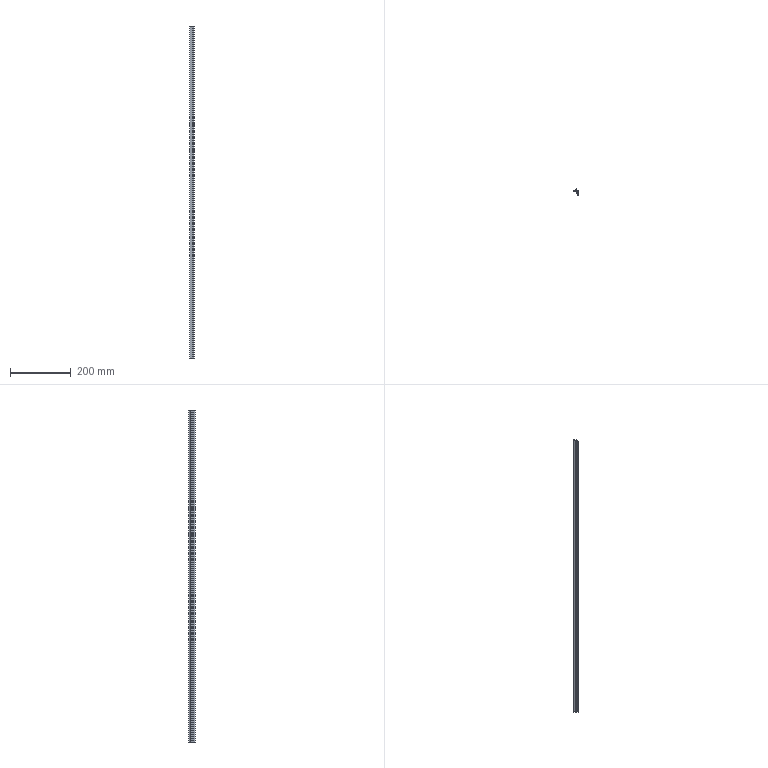Part | SolidWorks | features BaseBody 1, ICE 1, MoveFace 1 | 1 solid | 27 faces | box 14 x 20.3 x 1090 mm | volume 55498 mm3 | plane 20 | cylinder 7 | commonest cylinder face diameters 0.387 x2 0.8 x2 0.4 x1 20 x1 22 x1
STEP:
#1=CARTESIAN_POINT('',(-5.304,-0.625,200.));
#2=VERTEX_POINT('',#1);
#3=CARTESIAN_POINT('',(-5.449,-0.8125,200.));
#4=VERTEX_POINT('',#3);
#5=CARTESIAN_POINT('',(-5.255,-0.8125,200.));
#6=DIRECTION('',(0.,0.,1.));
#7=DIRECTION('',(-1.,0.,0.));
#8=AXIS2_PLACEMENT_3D('',#5,#6,#7);
#9=CIRCLE('',#8,0.1937);
#10=EDGE_CURVE('',#2,#4,#9,.T.);
#11=ORIENTED_EDGE('',*,*,#10,.T.);
#12=CARTESIAN_POINT('',(-5.449,-0.8125,-890.));
#13=VERTEX_POINT('',#12);
#14=CARTESIAN_POINT('',(-5.449,-0.8125,230.));
#15=DIRECTION('',(0.,0.,-1.));
#16=VECTOR('',#15,1000.);
#17=LINE('',#14,#16);
#18=EDGE_CURVE('',#4,#13,#17,.T.);
#19=ORIENTED_EDGE('',*,*,#18,.T.);
#20=CARTESIAN_POINT('',(-5.304,-0.625,-890.));
#21=VERTEX_POINT('',#20);
#22=CARTESIAN_POINT('',(-5.255,-0.8125,-890.));
#23=DIRECTION('',(0.,0.,-1.));
#24=DIRECTION('',(1.,0.,0.));
#25=AXIS2_PLACEMENT_3D('',#22,#23,#24);
#26=CIRCLE('',#25,0.1937);
#27=EDGE_CURVE('',#13,#21,#26,.T.);
#28=ORIENTED_EDGE('',*,*,#27,.T.);
#29=CARTESIAN_POINT('',(-5.304,-0.625,230.));
#30=DIRECTION('',(0.,0.,-1.));
#31=VECTOR('',#30,1000.);
#32=LINE('',#29,#31);
#33=EDGE_CURVE('',#2,#21,#32,.T.);
#34=ORIENTED_EDGE('',*,*,#33,.F.);
#35=EDGE_LOOP('',(#11,#19,#28,#34));
#36=FACE_OUTER_BOUND('',#35,.T.);
#37=CARTESIAN_POINT('',(-5.255,-0.8125,230.));
#38=DIRECTION('',(0.,0.,-1.));
#39=DIRECTION('',(-1.,0.,0.));
#40=AXIS2_PLACEMENT_3D('',#37,#38,#39);
#41=CYLINDRICAL_SURFACE('',#40,0.1937);
#42=ADVANCED_FACE('',(#36),#41,.F.);
#43=CARTESIAN_POINT('',(5.,-1.,-890.));
#44=VERTEX_POINT('',#43);
#45=CARTESIAN_POINT('',(5.,-14.3,-890.));
#46=VERTEX_POINT('',#45);
#47=CARTESIAN_POINT('',(5.,29.623,-890.));
#48=DIRECTION('',(0.,-1.,0.));
#49=VECTOR('',#48,1000.);
#50=LINE('',#47,#49);
#51=EDGE_CURVE('',#44,#46,#50,.T.);
#52=ORIENTED_EDGE('',*,*,#51,.F.);
#53=CARTESIAN_POINT('',(5.,-1.,200.));
#54=VERTEX_POINT('',#53);
#55=CARTESIAN_POINT('',(5.,-1.,230.));
#56=DIRECTION('',(0.,0.,-1.));
#57=VECTOR('',#56,1000.);
#58=LINE('',#55,#57);
#59=EDGE_CURVE('',#54,#44,#58,.T.);
#60=ORIENTED_EDGE('',*,*,#59,.F.);
#61=CARTESIAN_POINT('',(5.,-14.3,200.));
#62=VERTEX_POINT('',#61);
#63=CARTESIAN_POINT('',(5.,-14.3,200.));
#64=DIRECTION('',(0.,1.,0.));
#65=VECTOR('',#64,1000.);
#66=LINE('',#63,#65);
#67=EDGE_CURVE('',#62,#54,#66,.T.);
#68=ORIENTED_EDGE('',*,*,#67,.F.);
#69=CARTESIAN_POINT('',(5.,-14.3,230.));
#70=DIRECTION('',(0.,0.,1.));
#71=VECTOR('',#70,1000.);
#72=LINE('',#69,#71);
#73=EDGE_CURVE('',#46,#62,#72,.T.);
#74=ORIENTED_EDGE('',*,*,#73,.F.);
#75=EDGE_LOOP('',(#52,#60,#68,#74));
#76=FACE_OUTER_BOUND('',#75,.T.);
#77=CARTESIAN_POINT('',(5.,-14.3,230.));
#78=DIRECTION('',(-1.,0.,0.));
#79=DIRECTION('',(0.,0.,1.));
#80=AXIS2_PLACEMENT_3D('',#77,#78,#79);
#81=PLANE('',#80);
#82=ADVANCED_FACE('',(#76),#81,.F.);
#83=CARTESIAN_POINT('',(-9.,-2.,-890.));
#84=VERTEX_POINT('',#83);
#85=CARTESIAN_POINT('',(-9.,-2.,200.));
#86=VERTEX_POINT('',#85);
#87=CARTESIAN_POINT('',(-9.,-2.,230.));
#88=DIRECTION('',(0.,0.,1.));
#89=VECTOR('',#88,1000.);
#90=LINE('',#87,#89);
#91=EDGE_CURVE('',#84,#86,#90,.T.);
#92=ORIENTED_EDGE('',*,*,#91,.F.);
#93=CARTESIAN_POINT('',(0.9,-2.,-890.));
#94=VERTEX_POINT('',#93);
#95=CARTESIAN_POINT('',(5.,-2.,-890.));
#96=DIRECTION('',(-1.,0.,0.));
#97=VECTOR('',#96,1000.);
#98=LINE('',#95,#97);
#99=EDGE_CURVE('',#94,#84,#98,.T.);
#100=ORIENTED_EDGE('',*,*,#99,.F.);
#101=CARTESIAN_POINT('',(0.9,-2.,200.));
#102=VERTEX_POINT('',#101);
#103=CARTESIAN_POINT('',(0.9,-2.,230.));
#104=DIRECTION('',(0.,0.,-1.));
#105=VECTOR('',#104,1000.);
#106=LINE('',#103,#105);
#107=EDGE_CURVE('',#102,#94,#106,.T.);
#108=ORIENTED_EDGE('',*,*,#107,.F.);
#109=CARTESIAN_POINT('',(5.,-2.,200.));
#110=DIRECTION('',(1.,0.,0.));
#111=VECTOR('',#110,1000.);
#112=LINE('',#109,#111);
#113=EDGE_CURVE('',#86,#102,#112,.T.);
#114=ORIENTED_EDGE('',*,*,#113,.F.);
#115=EDGE_LOOP('',(#92,#100,#108,#114));
#116=FACE_OUTER_BOUND('',#115,.T.);
#117=CARTESIAN_POINT('',(-9.,-2.,230.));
#118=DIRECTION('',(0.,1.,0.));
#119=DIRECTION('',(0.,0.,1.));
#120=AXIS2_PLACEMENT_3D('',#117,#118,#119);
#121=PLANE('',#120);
#122=ADVANCED_FACE('',(#116),#121,.F.);
#123=CARTESIAN_POINT('',(4.,-6.,200.));
#124=VERTEX_POINT('',#123);
#125=CARTESIAN_POINT('',(4.,-3.,200.));
#126=VERTEX_POINT('',#125);
#127=CARTESIAN_POINT('',(4.,29.623,200.));
#128=DIRECTION('',(0.,1.,0.));
#129=VECTOR('',#128,1000.);
#130=LINE('',#127,#129);
#131=EDGE_CURVE('',#124,#126,#130,.T.);
#132=ORIENTED_EDGE('',*,*,#131,.F.);
#133=CARTESIAN_POINT('',(1.,-6.,200.));
#134=VERTEX_POINT('',#133);
#135=CARTESIAN_POINT('',(5.,-6.,200.));
#136=DIRECTION('',(1.,0.,0.));
#137=VECTOR('',#136,1000.);
#138=LINE('',#135,#137);
#139=EDGE_CURVE('',#134,#124,#138,.T.);
#140=ORIENTED_EDGE('',*,*,#139,.F.);
#141=CARTESIAN_POINT('',(1.,-6.7,200.));
#142=VERTEX_POINT('',#141);
#143=CARTESIAN_POINT('',(1.,-6.,200.));
#144=DIRECTION('',(0.,-1.,0.));
#145=VECTOR('',#144,1000.);
#146=LINE('',#143,#145);
#147=EDGE_CURVE('',#134,#142,#146,.T.);
#148=ORIENTED_EDGE('',*,*,#147,.T.);
#149=CARTESIAN_POINT('',(-1.7,-6.7,200.));
#150=VERTEX_POINT('',#149);
#151=CARTESIAN_POINT('',(5.,-6.7,200.));
#152=DIRECTION('',(1.,0.,0.));
#153=VECTOR('',#152,1000.);
#154=LINE('',#151,#153);
#155=EDGE_CURVE('',#150,#142,#154,.T.);
#156=ORIENTED_EDGE('',*,*,#155,.F.);
#157=CARTESIAN_POINT('',(-1.7,-7.7,200.));
#158=VERTEX_POINT('',#157);
#159=CARTESIAN_POINT('',(-1.7,-6.7,200.));
#160=DIRECTION('',(0.,-1.,0.));
#161=VECTOR('',#160,1000.);
#162=LINE('',#159,#161);
#163=EDGE_CURVE('',#150,#158,#162,.T.);
#164=ORIENTED_EDGE('',*,*,#163,.T.);
#165=CARTESIAN_POINT('',(4.,-7.7,200.));
#166=VERTEX_POINT('',#165);
#167=CARTESIAN_POINT('',(5.,-7.7,200.));
#168=DIRECTION('',(-1.,0.,0.));
#169=VECTOR('',#168,1000.);
#170=LINE('',#167,#169);
#171=EDGE_CURVE('',#166,#158,#170,.T.);
#172=ORIENTED_EDGE('',*,*,#171,.F.);
#173=CARTESIAN_POINT('',(4.,-14.3,200.));
#174=VERTEX_POINT('',#173);
#175=CARTESIAN_POINT('',(4.,29.623,200.));
#176=DIRECTION('',(0.,1.,0.));
#177=VECTOR('',#176,1000.);
#178=LINE('',#175,#177);
#179=EDGE_CURVE('',#174,#166,#178,.T.);
#180=ORIENTED_EDGE('',*,*,#179,.F.);
#181=CARTESIAN_POINT('',(5.,-14.3,200.));
#182=DIRECTION('',(-1.,0.,0.));
#183=VECTOR('',#182,1000.);
#184=LINE('',#181,#183);
#185=EDGE_CURVE('',#62,#174,#184,.T.);
#186=ORIENTED_EDGE('',*,*,#185,.F.);
#187=ORIENTED_EDGE('',*,*,#67,.T.);
#188=CARTESIAN_POINT('',(-5.207,-1.,200.));
#189=VERTEX_POINT('',#188);
#190=CARTESIAN_POINT('',(5.,-1.,200.));
#191=DIRECTION('',(1.,0.,0.));
#192=VECTOR('',#191,1000.);
#193=LINE('',#190,#192);
#194=EDGE_CURVE('',#189,#54,#193,.T.);
#195=ORIENTED_EDGE('',*,*,#194,.F.);
#196=CARTESIAN_POINT('',(-5.255,-0.8125,200.));
#197=DIRECTION('',(0.,0.,1.));
#198=DIRECTION('',(-1.,0.,0.));
#199=AXIS2_PLACEMENT_3D('',#196,#197,#198);
#200=CIRCLE('',#199,0.1937);
#201=EDGE_CURVE('',#4,#189,#200,.T.);
#202=ORIENTED_EDGE('',*,*,#201,.F.);
#203=ORIENTED_EDGE('',*,*,#10,.F.);
#204=CARTESIAN_POINT('',(-1.368,3.063,200.));
#205=VERTEX_POINT('',#204);
#206=CARTESIAN_POINT('',(-10.628,9.,200.));
#207=DIRECTION('',(0.,0.,1.));
#208=DIRECTION('',(-1.,0.,0.));
#209=AXIS2_PLACEMENT_3D('',#206,#207,#208);
#210=CIRCLE('',#209,11.);
#211=EDGE_CURVE('',#2,#205,#210,.T.);
#212=ORIENTED_EDGE('',*,*,#211,.T.);
#213=CARTESIAN_POINT('',(-1.,2.955,200.));
#214=VERTEX_POINT('',#213);
#215=CARTESIAN_POINT('',(-1.2,2.955,200.));
#216=DIRECTION('',(0.,0.,1.));
#217=DIRECTION('',(-1.,0.,0.));
#218=AXIS2_PLACEMENT_3D('',#215,#216,#217);
#219=CIRCLE('',#218,0.2);
#220=EDGE_CURVE('',#214,#205,#219,.T.);
#221=ORIENTED_EDGE('',*,*,#220,.F.);
#222=CARTESIAN_POINT('',(-1.,1.5,200.));
#223=VERTEX_POINT('',#222);
#224=CARTESIAN_POINT('',(-1.,2.955,200.));
#225=DIRECTION('',(0.,1.,0.));
#226=VECTOR('',#225,1000.);
#227=LINE('',#224,#226);
#228=EDGE_CURVE('',#223,#214,#227,.T.);
#229=ORIENTED_EDGE('',*,*,#228,.F.);
#230=CARTESIAN_POINT('',(0.,1.5,200.));
#231=VERTEX_POINT('',#230);
#232=CARTESIAN_POINT('',(-1.,1.5,200.));
#233=DIRECTION('',(-1.,0.,0.));
#234=VECTOR('',#233,1000.);
#235=LINE('',#232,#234);
#236=EDGE_CURVE('',#231,#223,#235,.T.);
#237=ORIENTED_EDGE('',*,*,#236,.F.);
#238=CARTESIAN_POINT('',(0.,6.,200.));
#239=VERTEX_POINT('',#238);
#240=CARTESIAN_POINT('',(0.,1.5,200.));
#241=DIRECTION('',(0.,-1.,0.));
#242=VECTOR('',#241,1000.);
#243=LINE('',#240,#242);
#244=EDGE_CURVE('',#239,#231,#243,.T.);
#245=ORIENTED_EDGE('',*,*,#244,.F.);
#246=CARTESIAN_POINT('',(-0.8,6.,200.));
#247=VERTEX_POINT('',#246);
#248=CARTESIAN_POINT('',(0.,6.,200.));
#249=DIRECTION('',(1.,0.,0.));
#250=VECTOR('',#249,1000.);
#251=LINE('',#248,#250);
#252=EDGE_CURVE('',#247,#239,#251,.T.);
#253=ORIENTED_EDGE('',*,*,#252,.F.);
#254=CARTESIAN_POINT('',(-1.178,5.731,200.));
#255=VERTEX_POINT('',#254);
#256=CARTESIAN_POINT('',(-0.8,5.6,200.));
#257=DIRECTION('',(0.,0.,1.));
#258=DIRECTION('',(-1.,0.,0.));
#259=AXIS2_PLACEMENT_3D('',#256,#257,#258);
#260=CIRCLE('',#259,0.4);
#261=EDGE_CURVE('',#247,#255,#260,.T.);
#262=ORIENTED_EDGE('',*,*,#261,.T.);
#263=CARTESIAN_POINT('',(-8.678,-0.8077,200.));
#264=VERTEX_POINT('',#263);
#265=CARTESIAN_POINT('',(-10.628,9.,200.));
#266=DIRECTION('',(0.,0.,1.));
#267=DIRECTION('',(-1.,0.,0.));
#268=AXIS2_PLACEMENT_3D('',#265,#266,#267);
#269=CIRCLE('',#268,10.);
#270=EDGE_CURVE('',#264,#255,#269,.T.);
#271=ORIENTED_EDGE('',*,*,#270,.F.);
#272=CARTESIAN_POINT('',(-9.,-1.2,200.));
#273=VERTEX_POINT('',#272);
#274=CARTESIAN_POINT('',(-8.6,-1.2,200.));
#275=DIRECTION('',(0.,0.,1.));
#276=DIRECTION('',(-1.,0.,0.));
#277=AXIS2_PLACEMENT_3D('',#274,#275,#276);
#278=CIRCLE('',#277,0.4);
#279=EDGE_CURVE('',#264,#273,#278,.T.);
#280=ORIENTED_EDGE('',*,*,#279,.T.);
#281=CARTESIAN_POINT('',(-9.,8.,200.));
#282=DIRECTION('',(0.,-1.,0.));
#283=VECTOR('',#282,1000.);
#284=LINE('',#281,#283);
#285=EDGE_CURVE('',#273,#86,#284,.T.);
#286=ORIENTED_EDGE('',*,*,#285,.T.);
#287=ORIENTED_EDGE('',*,*,#113,.T.);
#288=CARTESIAN_POINT('',(0.9,-3.,200.));
#289=VERTEX_POINT('',#288);
#290=CARTESIAN_POINT('',(0.9,29.623,200.));
#291=DIRECTION('',(0.,1.,0.));
#292=VECTOR('',#291,1000.);
#293=LINE('',#290,#292);
#294=EDGE_CURVE('',#289,#102,#293,.T.);
#295=ORIENTED_EDGE('',*,*,#294,.F.);
#296=CARTESIAN_POINT('',(5.,-3.,200.));
#297=DIRECTION('',(-1.,0.,0.));
#298=VECTOR('',#297,1000.);
#299=LINE('',#296,#298);
#300=EDGE_CURVE('',#126,#289,#299,.T.);
#301=ORIENTED_EDGE('',*,*,#300,.F.);
#302=EDGE_LOOP('',(#132,#140,#148,#156,#164,#172,#180,#186,#187,#195,#202,#203,#212,#221,#229,#237,#245,#253,#262,#271,#280,#286,#287,#295,#301));
#303=FACE_OUTER_BOUND('',#302,.T.);
#304=CARTESIAN_POINT('',(5.,29.623,200.));
#305=DIRECTION('',(0.,0.,-1.));
#306=DIRECTION('',(-1.,0.,0.));
#307=AXIS2_PLACEMENT_3D('',#304,#305,#306);
#308=PLANE('',#307);
#309=ADVANCED_FACE('',(#303),#308,.F.);
#310=ORIENTED_EDGE('',*,*,#185,.T.);
#311=CARTESIAN_POINT('',(4.,-14.3,-890.));
#312=VERTEX_POINT('',#311);
#313=CARTESIAN_POINT('',(4.,-14.3,230.));
#314=DIRECTION('',(0.,0.,1.));
#315=VECTOR('',#314,1000.);
#316=LINE('',#313,#315);
#317=EDGE_CURVE('',#312,#174,#316,.T.);
#318=ORIENTED_EDGE('',*,*,#317,.F.);
#319=CARTESIAN_POINT('',(5.,-14.3,-890.));
#320=DIRECTION('',(-1.,0.,0.));
#321=VECTOR('',#320,1000.);
#322=LINE('',#319,#321);
#323=EDGE_CURVE('',#46,#312,#322,.T.);
#324=ORIENTED_EDGE('',*,*,#323,.F.);
#325=ORIENTED_EDGE('',*,*,#73,.T.);
#326=EDGE_LOOP('',(#310,#318,#324,#325));
#327=FACE_OUTER_BOUND('',#326,.T.);
#328=CARTESIAN_POINT('',(4.,-14.3,230.));
#329=DIRECTION('',(0.,1.,0.));
#330=DIRECTION('',(0.,0.,1.));
#331=AXIS2_PLACEMENT_3D('',#328,#329,#330);
#332=PLANE('',#331);
#333=ADVANCED_FACE('',(#327),#332,.F.);
#334=ORIENTED_EDGE('',*,*,#51,.T.);
#335=ORIENTED_EDGE('',*,*,#323,.T.);
#336=CARTESIAN_POINT('',(4.,-7.7,-890.));
#337=VERTEX_POINT('',#336);
#338=CARTESIAN_POINT('',(4.,-7.7,-890.));
#339=DIRECTION('',(0.,-1.,0.));
#340=VECTOR('',#339,1000.);
#341=LINE('',#338,#340);
#342=EDGE_CURVE('',#337,#312,#341,.T.);
#343=ORIENTED_EDGE('',*,*,#342,.F.);
#344=CARTESIAN_POINT('',(-1.7,-7.7,-890.));
#345=VERTEX_POINT('',#344);
#346=CARTESIAN_POINT('',(-1.7,-7.7,-890.));
#347=DIRECTION('',(1.,0.,0.));
#348=VECTOR('',#347,1000.);
#349=LINE('',#346,#348);
#350=EDGE_CURVE('',#345,#337,#349,.T.);
#351=ORIENTED_EDGE('',*,*,#350,.F.);
#352=CARTESIAN_POINT('',(-1.7,-6.7,-890.));
#353=VERTEX_POINT('',#352);
#354=CARTESIAN_POINT('',(-1.7,29.623,-890.));
#355=DIRECTION('',(0.,1.,0.));
#356=VECTOR('',#355,1000.);
#357=LINE('',#354,#356);
#358=EDGE_CURVE('',#345,#353,#357,.T.);
#359=ORIENTED_EDGE('',*,*,#358,.T.);
#360=CARTESIAN_POINT('',(1.,-6.7,-890.));
#361=VERTEX_POINT('',#360);
#362=CARTESIAN_POINT('',(1.,-6.7,-890.));
#363=DIRECTION('',(-1.,0.,0.));
#364=VECTOR('',#363,1000.);
#365=LINE('',#362,#364);
#366=EDGE_CURVE('',#361,#353,#365,.T.);
#367=ORIENTED_EDGE('',*,*,#366,.F.);
#368=CARTESIAN_POINT('',(1.,-6.,-890.));
#369=VERTEX_POINT('',#368);
#370=CARTESIAN_POINT('',(1.,29.623,-890.));
#371=DIRECTION('',(0.,1.,0.));
#372=VECTOR('',#371,1000.);
#373=LINE('',#370,#372);
#374=EDGE_CURVE('',#361,#369,#373,.T.);
#375=ORIENTED_EDGE('',*,*,#374,.T.);
#376=CARTESIAN_POINT('',(4.,-6.,-890.));
#377=VERTEX_POINT('',#376);
#378=CARTESIAN_POINT('',(4.,-6.,-890.));
#379=DIRECTION('',(-1.,0.,0.));
#380=VECTOR('',#379,1000.);
#381=LINE('',#378,#380);
#382=EDGE_CURVE('',#377,#369,#381,.T.);
#383=ORIENTED_EDGE('',*,*,#382,.F.);
#384=CARTESIAN_POINT('',(4.,-3.,-890.));
#385=VERTEX_POINT('',#384);
#386=CARTESIAN_POINT('',(4.,-3.,-890.));
#387=DIRECTION('',(0.,-1.,0.));
#388=VECTOR('',#387,1000.);
#389=LINE('',#386,#388);
#390=EDGE_CURVE('',#385,#377,#389,.T.);
#391=ORIENTED_EDGE('',*,*,#390,.F.);
#392=CARTESIAN_POINT('',(0.9,-3.,-890.));
#393=VERTEX_POINT('',#392);
#394=CARTESIAN_POINT('',(0.9,-3.,-890.));
#395=DIRECTION('',(1.,0.,0.));
#396=VECTOR('',#395,1000.);
#397=LINE('',#394,#396);
#398=EDGE_CURVE('',#393,#385,#397,.T.);
#399=ORIENTED_EDGE('',*,*,#398,.F.);
#400=CARTESIAN_POINT('',(0.9,-2.,-890.));
#401=DIRECTION('',(0.,-1.,0.));
#402=VECTOR('',#401,1000.);
#403=LINE('',#400,#402);
#404=EDGE_CURVE('',#94,#393,#403,.T.);
#405=ORIENTED_EDGE('',*,*,#404,.F.);
#406=ORIENTED_EDGE('',*,*,#99,.T.);
#407=CARTESIAN_POINT('',(-9.,-1.2,-890.));
#408=VERTEX_POINT('',#407);
#409=CARTESIAN_POINT('',(-9.,-1.2,-890.));
#410=DIRECTION('',(0.,-1.,0.));
#411=VECTOR('',#410,1000.);
#412=LINE('',#409,#411);
#413=EDGE_CURVE('',#408,#84,#412,.T.);
#414=ORIENTED_EDGE('',*,*,#413,.F.);
#415=CARTESIAN_POINT('',(-8.678,-0.8077,-890.));
#416=VERTEX_POINT('',#415);
#417=CARTESIAN_POINT('',(-8.6,-1.2,-890.));
#418=DIRECTION('',(0.,0.,-1.));
#419=DIRECTION('',(1.,0.,0.));
#420=AXIS2_PLACEMENT_3D('',#417,#418,#419);
#421=CIRCLE('',#420,0.4);
#422=EDGE_CURVE('',#408,#416,#421,.T.);
#423=ORIENTED_EDGE('',*,*,#422,.T.);
#424=CARTESIAN_POINT('',(-1.178,5.731,-890.));
#425=VERTEX_POINT('',#424);
#426=CARTESIAN_POINT('',(-10.628,9.,-890.));
#427=DIRECTION('',(0.,0.,-1.));
#428=DIRECTION('',(1.,0.,0.));
#429=AXIS2_PLACEMENT_3D('',#426,#427,#428);
#430=CIRCLE('',#429,10.);
#431=EDGE_CURVE('',#425,#416,#430,.T.);
#432=ORIENTED_EDGE('',*,*,#431,.F.);
#433=CARTESIAN_POINT('',(-0.8,6.,-890.));
#434=VERTEX_POINT('',#433);
#435=CARTESIAN_POINT('',(-0.8,5.6,-890.));
#436=DIRECTION('',(0.,0.,-1.));
#437=DIRECTION('',(1.,0.,0.));
#438=AXIS2_PLACEMENT_3D('',#435,#436,#437);
#439=CIRCLE('',#438,0.4);
#440=EDGE_CURVE('',#425,#434,#439,.T.);
#441=ORIENTED_EDGE('',*,*,#440,.T.);
#442=CARTESIAN_POINT('',(0.,6.,-890.));
#443=VERTEX_POINT('',#442);
#444=CARTESIAN_POINT('',(0.,6.,-890.));
#445=DIRECTION('',(-1.,0.,0.));
#446=VECTOR('',#445,1000.);
#447=LINE('',#444,#446);
#448=EDGE_CURVE('',#443,#434,#447,.T.);
#449=ORIENTED_EDGE('',*,*,#448,.F.);
#450=CARTESIAN_POINT('',(0.,1.5,-890.));
#451=VERTEX_POINT('',#450);
#452=CARTESIAN_POINT('',(0.,1.5,-890.));
#453=DIRECTION('',(0.,1.,0.));
#454=VECTOR('',#453,1000.);
#455=LINE('',#452,#454);
#456=EDGE_CURVE('',#451,#443,#455,.T.);
#457=ORIENTED_EDGE('',*,*,#456,.F.);
#458=CARTESIAN_POINT('',(-1.,1.5,-890.));
#459=VERTEX_POINT('',#458);
#460=CARTESIAN_POINT('',(-1.,1.5,-890.));
#461=DIRECTION('',(1.,0.,0.));
#462=VECTOR('',#461,1000.);
#463=LINE('',#460,#462);
#464=EDGE_CURVE('',#459,#451,#463,.T.);
#465=ORIENTED_EDGE('',*,*,#464,.F.);
#466=CARTESIAN_POINT('',(-1.,2.955,-890.));
#467=VERTEX_POINT('',#466);
#468=CARTESIAN_POINT('',(-1.,2.955,-890.));
#469=DIRECTION('',(0.,-1.,0.));
#470=VECTOR('',#469,1000.);
#471=LINE('',#468,#470);
#472=EDGE_CURVE('',#467,#459,#471,.T.);
#473=ORIENTED_EDGE('',*,*,#472,.F.);
#474=CARTESIAN_POINT('',(-1.368,3.063,-890.));
#475=VERTEX_POINT('',#474);
#476=CARTESIAN_POINT('',(-1.2,2.955,-890.));
#477=DIRECTION('',(0.,0.,-1.));
#478=DIRECTION('',(1.,0.,0.));
#479=AXIS2_PLACEMENT_3D('',#476,#477,#478);
#480=CIRCLE('',#479,0.2);
#481=EDGE_CURVE('',#475,#467,#480,.T.);
#482=ORIENTED_EDGE('',*,*,#481,.F.);
#483=CARTESIAN_POINT('',(-10.628,9.,-890.));
#484=DIRECTION('',(0.,0.,-1.));
#485=DIRECTION('',(1.,0.,0.));
#486=AXIS2_PLACEMENT_3D('',#483,#484,#485);
#487=CIRCLE('',#486,11.);
#488=EDGE_CURVE('',#475,#21,#487,.T.);
#489=ORIENTED_EDGE('',*,*,#488,.T.);
#490=ORIENTED_EDGE('',*,*,#27,.F.);
#491=CARTESIAN_POINT('',(-5.207,-1.,-890.));
#492=VERTEX_POINT('',#491);
#493=CARTESIAN_POINT('',(-5.255,-0.8125,-890.));
#494=DIRECTION('',(0.,0.,-1.));
#495=DIRECTION('',(1.,0.,0.));
#496=AXIS2_PLACEMENT_3D('',#493,#494,#495);
#497=CIRCLE('',#496,0.1937);
#498=EDGE_CURVE('',#492,#13,#497,.T.);
#499=ORIENTED_EDGE('',*,*,#498,.F.);
#500=CARTESIAN_POINT('',(5.,-1.,-890.));
#501=DIRECTION('',(-1.,0.,0.));
#502=VECTOR('',#501,1000.);
#503=LINE('',#500,#502);
#504=EDGE_CURVE('',#44,#492,#503,.T.);
#505=ORIENTED_EDGE('',*,*,#504,.F.);
#506=EDGE_LOOP('',(#334,#335,#343,#351,#359,#367,#375,#383,#391,#399,#405,#406,#414,#423,#432,#441,#449,#457,#465,#473,#482,#489,#490,#499,#505));
#507=FACE_OUTER_BOUND('',#506,.T.);
#508=CARTESIAN_POINT('',(5.,29.623,-890.));
#509=DIRECTION('',(0.,0.,1.));
#510=DIRECTION('',(1.,0.,0.));
#511=AXIS2_PLACEMENT_3D('',#508,#509,#510);
#512=PLANE('',#511);
#513=ADVANCED_FACE('',(#507),#512,.F.);
#514=ORIENTED_EDGE('',*,*,#59,.T.);
#515=ORIENTED_EDGE('',*,*,#504,.T.);
#516=CARTESIAN_POINT('',(-5.207,-1.,230.));
#517=DIRECTION('',(0.,0.,-1.));
#518=VECTOR('',#517,1000.);
#519=LINE('',#516,#518);
#520=EDGE_CURVE('',#189,#492,#519,.T.);
#521=ORIENTED_EDGE('',*,*,#520,.F.);
#522=ORIENTED_EDGE('',*,*,#194,.T.);
#523=EDGE_LOOP('',(#514,#515,#521,#522));
#524=FACE_OUTER_BOUND('',#523,.T.);
#525=CARTESIAN_POINT('',(5.,-1.,230.));
#526=DIRECTION('',(0.,-1.,0.));
#527=DIRECTION('',(0.,0.,-1.));
#528=AXIS2_PLACEMENT_3D('',#525,#526,#527);
#529=PLANE('',#528);
#530=ADVANCED_FACE('',(#524),#529,.F.);
#531=CARTESIAN_POINT('',(-9.,-1.2,230.));
#532=DIRECTION('',(0.,0.,1.));
#533=VECTOR('',#532,1000.);
#534=LINE('',#531,#533);
#535=EDGE_CURVE('',#408,#273,#534,.T.);
#536=ORIENTED_EDGE('',*,*,#535,.F.);
#537=ORIENTED_EDGE('',*,*,#413,.T.);
#538=ORIENTED_EDGE('',*,*,#91,.T.);
#539=ORIENTED_EDGE('',*,*,#285,.F.);
#540=EDGE_LOOP('',(#536,#537,#538,#539));
#541=FACE_OUTER_BOUND('',#540,.T.);
#542=CARTESIAN_POINT('',(-9.,-1.2,230.));
#543=DIRECTION('',(1.,0.,0.));
#544=DIRECTION('',(0.,0.,-1.));
#545=AXIS2_PLACEMENT_3D('',#542,#543,#544);
#546=PLANE('',#545);
#547=ADVANCED_FACE('',(#541),#546,.F.);
#548=ORIENTED_EDGE('',*,*,#294,.T.);
#549=ORIENTED_EDGE('',*,*,#107,.T.);
#550=ORIENTED_EDGE('',*,*,#404,.T.);
#551=CARTESIAN_POINT('',(0.9,-3.,230.));
#552=DIRECTION('',(0.,0.,-1.));
#553=VECTOR('',#552,1000.);
#554=LINE('',#551,#553);
#555=EDGE_CURVE('',#289,#393,#554,.T.);
#556=ORIENTED_EDGE('',*,*,#555,.F.);
#557=EDGE_LOOP('',(#548,#549,#550,#556));
#558=FACE_OUTER_BOUND('',#557,.T.);
#559=CARTESIAN_POINT('',(0.9,-2.,230.));
#560=DIRECTION('',(1.,0.,0.));
#561=DIRECTION('',(0.,0.,-1.));
#562=AXIS2_PLACEMENT_3D('',#559,#560,#561);
#563=PLANE('',#562);
#564=ADVANCED_FACE('',(#558),#563,.F.);
#565=ORIENTED_EDGE('',*,*,#300,.T.);
#566=ORIENTED_EDGE('',*,*,#555,.T.);
#567=ORIENTED_EDGE('',*,*,#398,.T.);
#568=CARTESIAN_POINT('',(4.,-3.,230.));
#569=DIRECTION('',(0.,0.,-1.));
#570=VECTOR('',#569,1000.);
#571=LINE('',#568,#570);
#572=EDGE_CURVE('',#126,#385,#571,.T.);
#573=ORIENTED_EDGE('',*,*,#572,.F.);
#574=EDGE_LOOP('',(#565,#566,#567,#573));
#575=FACE_OUTER_BOUND('',#574,.T.);
#576=CARTESIAN_POINT('',(0.9,-3.,230.));
#577=DIRECTION('',(0.,1.,0.));
#578=DIRECTION('',(0.,0.,1.));
#579=AXIS2_PLACEMENT_3D('',#576,#577,#578);
#580=PLANE('',#579);
#581=ADVANCED_FACE('',(#575),#580,.F.);
#582=ORIENTED_EDGE('',*,*,#131,.T.);
#583=ORIENTED_EDGE('',*,*,#572,.T.);
#584=ORIENTED_EDGE('',*,*,#390,.T.);
#585=CARTESIAN_POINT('',(4.,-6.,230.));
#586=DIRECTION('',(0.,0.,-1.));
#587=VECTOR('',#586,1000.);
#588=LINE('',#585,#587);
#589=EDGE_CURVE('',#124,#377,#588,.T.);
#590=ORIENTED_EDGE('',*,*,#589,.F.);
#591=EDGE_LOOP('',(#582,#583,#584,#590));
#592=FACE_OUTER_BOUND('',#591,.T.);
#593=CARTESIAN_POINT('',(4.,-3.,230.));
#594=DIRECTION('',(1.,0.,0.));
#595=DIRECTION('',(0.,0.,-1.));
#596=AXIS2_PLACEMENT_3D('',#593,#594,#595);
#597=PLANE('',#596);
#598=ADVANCED_FACE('',(#592),#597,.F.);
#599=ORIENTED_EDGE('',*,*,#139,.T.);
#600=ORIENTED_EDGE('',*,*,#589,.T.);
#601=ORIENTED_EDGE('',*,*,#382,.T.);
#602=CARTESIAN_POINT('',(1.,-6.,230.));
#603=DIRECTION('',(0.,0.,-1.));
#604=VECTOR('',#603,1000.);
#605=LINE('',#602,#604);
#606=EDGE_CURVE('',#134,#369,#605,.T.);
#607=ORIENTED_EDGE('',*,*,#606,.F.);
#608=EDGE_LOOP('',(#599,#600,#601,#607));
#609=FACE_OUTER_BOUND('',#608,.T.);
#610=CARTESIAN_POINT('',(4.,-6.,230.));
#611=DIRECTION('',(0.,-1.,0.));
#612=DIRECTION('',(0.,0.,-1.));
#613=AXIS2_PLACEMENT_3D('',#610,#611,#612);
#614=PLANE('',#613);
#615=ADVANCED_FACE('',(#609),#614,.F.);
#616=ORIENTED_EDGE('',*,*,#155,.T.);
#617=CARTESIAN_POINT('',(1.,-6.7,230.));
#618=DIRECTION('',(0.,0.,1.));
#619=VECTOR('',#618,1000.);
#620=LINE('',#617,#619);
#621=EDGE_CURVE('',#361,#142,#620,.T.);
#622=ORIENTED_EDGE('',*,*,#621,.F.);
#623=ORIENTED_EDGE('',*,*,#366,.T.);
#624=CARTESIAN_POINT('',(-1.7,-6.7,230.));
#625=DIRECTION('',(0.,0.,-1.));
#626=VECTOR('',#625,1000.);
#627=LINE('',#624,#626);
#628=EDGE_CURVE('',#150,#353,#627,.T.);
#629=ORIENTED_EDGE('',*,*,#628,.F.);
#630=EDGE_LOOP('',(#616,#622,#623,#629));
#631=FACE_OUTER_BOUND('',#630,.T.);
#632=CARTESIAN_POINT('',(1.,-6.7,230.));
#633=DIRECTION('',(0.,-1.,0.));
#634=DIRECTION('',(0.,0.,-1.));
#635=AXIS2_PLACEMENT_3D('',#632,#633,#634);
#636=PLANE('',#635);
#637=ADVANCED_FACE('',(#631),#636,.F.);
#638=ORIENTED_EDGE('',*,*,#171,.T.);
#639=CARTESIAN_POINT('',(-1.7,-7.7,230.));
#640=DIRECTION('',(0.,0.,1.));
#641=VECTOR('',#640,1000.);
#642=LINE('',#639,#641);
#643=EDGE_CURVE('',#345,#158,#642,.T.);
#644=ORIENTED_EDGE('',*,*,#643,.F.);
#645=ORIENTED_EDGE('',*,*,#350,.T.);
#646=CARTESIAN_POINT('',(4.,-7.7,230.));
#647=DIRECTION('',(0.,0.,-1.));
#648=VECTOR('',#647,1000.);
#649=LINE('',#646,#648);
#650=EDGE_CURVE('',#166,#337,#649,.T.);
#651=ORIENTED_EDGE('',*,*,#650,.F.);
#652=EDGE_LOOP('',(#638,#644,#645,#651));
#653=FACE_OUTER_BOUND('',#652,.T.);
#654=CARTESIAN_POINT('',(-1.7,-7.7,230.));
#655=DIRECTION('',(0.,1.,0.));
#656=DIRECTION('',(0.,0.,1.));
#657=AXIS2_PLACEMENT_3D('',#654,#655,#656);
#658=PLANE('',#657);
#659=ADVANCED_FACE('',(#653),#658,.F.);
#660=ORIENTED_EDGE('',*,*,#179,.T.);
#661=ORIENTED_EDGE('',*,*,#650,.T.);
#662=ORIENTED_EDGE('',*,*,#342,.T.);
#663=ORIENTED_EDGE('',*,*,#317,.T.);
#664=EDGE_LOOP('',(#660,#661,#662,#663));
#665=FACE_OUTER_BOUND('',#664,.T.);
#666=CARTESIAN_POINT('',(4.,-7.7,230.));
#667=DIRECTION('',(1.,0.,0.));
#668=DIRECTION('',(0.,0.,-1.));
#669=AXIS2_PLACEMENT_3D('',#666,#667,#668);
#670=PLANE('',#669);
#671=ADVANCED_FACE('',(#665),#670,.F.);
#672=ORIENTED_EDGE('',*,*,#18,.F.);
#673=ORIENTED_EDGE('',*,*,#201,.T.);
#674=ORIENTED_EDGE('',*,*,#520,.T.);
#675=ORIENTED_EDGE('',*,*,#498,.T.);
#676=EDGE_LOOP('',(#672,#673,#674,#675));
#677=FACE_OUTER_BOUND('',#676,.T.);
#678=CARTESIAN_POINT('',(-5.255,-0.8125,230.));
#679=DIRECTION('',(0.,0.,-1.));
#680=DIRECTION('',(-1.,0.,0.));
#681=AXIS2_PLACEMENT_3D('',#678,#679,#680);
#682=CYLINDRICAL_SURFACE('',#681,0.1937);
#683=ADVANCED_FACE('',(#677),#682,.F.);
#684=CARTESIAN_POINT('',(-1.,2.955,230.));
#685=DIRECTION('',(0.,0.,1.));
#686=VECTOR('',#685,1000.);
#687=LINE('',#684,#686);
#688=EDGE_CURVE('',#467,#214,#687,.T.);
#689=ORIENTED_EDGE('',*,*,#688,.F.);
#690=ORIENTED_EDGE('',*,*,#472,.T.);
#691=CARTESIAN_POINT('',(-1.,1.5,230.));
#692=DIRECTION('',(0.,0.,-1.));
#693=VECTOR('',#692,1000.);
#694=LINE('',#691,#693);
#695=EDGE_CURVE('',#223,#459,#694,.T.);
#696=ORIENTED_EDGE('',*,*,#695,.F.);
#697=ORIENTED_EDGE('',*,*,#228,.T.);
#698=EDGE_LOOP('',(#689,#690,#696,#697));
#699=FACE_OUTER_BOUND('',#698,.T.);
#700=CARTESIAN_POINT('',(-1.,2.955,230.));
#701=DIRECTION('',(1.,0.,0.));
#702=DIRECTION('',(0.,0.,-1.));
#703=AXIS2_PLACEMENT_3D('',#700,#701,#702);
#704=PLANE('',#703);
#705=ADVANCED_FACE('',(#699),#704,.F.);
#706=ORIENTED_EDGE('',*,*,#488,.F.);
#707=CARTESIAN_POINT('',(-1.368,3.063,230.));
#708=DIRECTION('',(0.,0.,1.));
#709=VECTOR('',#708,1000.);
#710=LINE('',#707,#709);
#711=EDGE_CURVE('',#475,#205,#710,.T.);
#712=ORIENTED_EDGE('',*,*,#711,.T.);
#713=ORIENTED_EDGE('',*,*,#211,.F.);
#714=ORIENTED_EDGE('',*,*,#33,.T.);
#715=EDGE_LOOP('',(#706,#712,#713,#714));
#716=FACE_OUTER_BOUND('',#715,.T.);
#717=CARTESIAN_POINT('',(-10.628,9.,230.));
#718=DIRECTION('',(0.,0.,-1.));
#719=DIRECTION('',(-1.,0.,0.));
#720=AXIS2_PLACEMENT_3D('',#717,#718,#719);
#721=CYLINDRICAL_SURFACE('',#720,11.);
#722=ADVANCED_FACE('',(#716),#721,.T.);
#723=CARTESIAN_POINT('',(-1.178,5.731,230.));
#724=DIRECTION('',(0.,0.,1.));
#725=VECTOR('',#724,1000.);
#726=LINE('',#723,#725);
#727=EDGE_CURVE('',#425,#255,#726,.T.);
#728=ORIENTED_EDGE('',*,*,#727,.F.);
#729=ORIENTED_EDGE('',*,*,#431,.T.);
#730=CARTESIAN_POINT('',(-8.678,-0.8077,230.));
#731=DIRECTION('',(0.,0.,-1.));
#732=VECTOR('',#731,1000.);
#733=LINE('',#730,#732);
#734=EDGE_CURVE('',#264,#416,#733,.T.);
#735=ORIENTED_EDGE('',*,*,#734,.F.);
#736=ORIENTED_EDGE('',*,*,#270,.T.);
#737=EDGE_LOOP('',(#728,#729,#735,#736));
#738=FACE_OUTER_BOUND('',#737,.T.);
#739=CARTESIAN_POINT('',(-10.628,9.,230.));
#740=DIRECTION('',(0.,0.,-1.));
#741=DIRECTION('',(-1.,0.,0.));
#742=AXIS2_PLACEMENT_3D('',#739,#740,#741);
#743=CYLINDRICAL_SURFACE('',#742,10.);
#744=ADVANCED_FACE('',(#738),#743,.F.);
#745=CARTESIAN_POINT('',(0.,1.5,230.));
#746=DIRECTION('',(0.,0.,1.));
#747=VECTOR('',#746,1000.);
#748=LINE('',#745,#747);
#749=EDGE_CURVE('',#451,#231,#748,.T.);
#750=ORIENTED_EDGE('',*,*,#749,.F.);
#751=ORIENTED_EDGE('',*,*,#456,.T.);
#752=CARTESIAN_POINT('',(0.,6.,230.));
#753=DIRECTION('',(0.,0.,-1.));
#754=VECTOR('',#753,1000.);
#755=LINE('',#752,#754);
#756=EDGE_CURVE('',#239,#443,#755,.T.);
#757=ORIENTED_EDGE('',*,*,#756,.F.);
#758=ORIENTED_EDGE('',*,*,#244,.T.);
#759=EDGE_LOOP('',(#750,#751,#757,#758));
#760=FACE_OUTER_BOUND('',#759,.T.);
#761=CARTESIAN_POINT('',(0.,1.5,230.));
#762=DIRECTION('',(-1.,0.,0.));
#763=DIRECTION('',(0.,0.,1.));
#764=AXIS2_PLACEMENT_3D('',#761,#762,#763);
#765=PLANE('',#764);
#766=ADVANCED_FACE('',(#760),#765,.F.);
#767=ORIENTED_EDGE('',*,*,#422,.F.);
#768=ORIENTED_EDGE('',*,*,#535,.T.);
#769=ORIENTED_EDGE('',*,*,#279,.F.);
#770=ORIENTED_EDGE('',*,*,#734,.T.);
#771=EDGE_LOOP('',(#767,#768,#769,#770));
#772=FACE_OUTER_BOUND('',#771,.T.);
#773=CARTESIAN_POINT('',(-8.6,-1.2,230.));
#774=DIRECTION('',(0.,0.,-1.));
#775=DIRECTION('',(-1.,0.,0.));
#776=AXIS2_PLACEMENT_3D('',#773,#774,#775);
#777=CYLINDRICAL_SURFACE('',#776,0.4);
#778=ADVANCED_FACE('',(#772),#777,.T.);
#779=ORIENTED_EDGE('',*,*,#147,.F.);
#780=ORIENTED_EDGE('',*,*,#606,.T.);
#781=ORIENTED_EDGE('',*,*,#374,.F.);
#782=ORIENTED_EDGE('',*,*,#621,.T.);
#783=EDGE_LOOP('',(#779,#780,#781,#782));
#784=FACE_OUTER_BOUND('',#783,.T.);
#785=CARTESIAN_POINT('',(1.,-6.,230.));
#786=DIRECTION('',(1.,0.,0.));
#787=DIRECTION('',(0.,0.,-1.));
#788=AXIS2_PLACEMENT_3D('',#785,#786,#787);
#789=PLANE('',#788);
#790=ADVANCED_FACE('',(#784),#789,.F.);
#791=ORIENTED_EDGE('',*,*,#163,.F.);
#792=ORIENTED_EDGE('',*,*,#628,.T.);
#793=ORIENTED_EDGE('',*,*,#358,.F.);
#794=ORIENTED_EDGE('',*,*,#643,.T.);
#795=EDGE_LOOP('',(#791,#792,#793,#794));
#796=FACE_OUTER_BOUND('',#795,.T.);
#797=CARTESIAN_POINT('',(-1.7,-6.7,230.));
#798=DIRECTION('',(1.,0.,0.));
#799=DIRECTION('',(0.,0.,-1.));
#800=AXIS2_PLACEMENT_3D('',#797,#798,#799);
#801=PLANE('',#800);
#802=ADVANCED_FACE('',(#796),#801,.F.);
#803=ORIENTED_EDGE('',*,*,#711,.F.);
#804=ORIENTED_EDGE('',*,*,#481,.T.);
#805=ORIENTED_EDGE('',*,*,#688,.T.);
#806=ORIENTED_EDGE('',*,*,#220,.T.);
#807=EDGE_LOOP('',(#803,#804,#805,#806));
#808=FACE_OUTER_BOUND('',#807,.T.);
#809=CARTESIAN_POINT('',(-1.2,2.955,230.));
#810=DIRECTION('',(0.,0.,-1.));
#811=DIRECTION('',(-1.,0.,0.));
#812=AXIS2_PLACEMENT_3D('',#809,#810,#811);
#813=CYLINDRICAL_SURFACE('',#812,0.2);
#814=ADVANCED_FACE('',(#808),#813,.F.);
#815=ORIENTED_EDGE('',*,*,#695,.T.);
#816=ORIENTED_EDGE('',*,*,#464,.T.);
#817=ORIENTED_EDGE('',*,*,#749,.T.);
#818=ORIENTED_EDGE('',*,*,#236,.T.);
#819=EDGE_LOOP('',(#815,#816,#817,#818));
#820=FACE_OUTER_BOUND('',#819,.T.);
#821=CARTESIAN_POINT('',(-1.,1.5,230.));
#822=DIRECTION('',(0.,1.,0.));
#823=DIRECTION('',(0.,0.,1.));
#824=AXIS2_PLACEMENT_3D('',#821,#822,#823);
#825=PLANE('',#824);
#826=ADVANCED_FACE('',(#820),#825,.F.);
#827=ORIENTED_EDGE('',*,*,#440,.F.);
#828=ORIENTED_EDGE('',*,*,#727,.T.);
#829=ORIENTED_EDGE('',*,*,#261,.F.);
#830=CARTESIAN_POINT('',(-0.8,6.,230.));
#831=DIRECTION('',(0.,0.,-1.));
#832=VECTOR('',#831,1000.);
#833=LINE('',#830,#832);
#834=EDGE_CURVE('',#247,#434,#833,.T.);
#835=ORIENTED_EDGE('',*,*,#834,.T.);
#836=EDGE_LOOP('',(#827,#828,#829,#835));
#837=FACE_OUTER_BOUND('',#836,.T.);
#838=CARTESIAN_POINT('',(-0.8,5.6,230.));
#839=DIRECTION('',(0.,0.,-1.));
#840=DIRECTION('',(-1.,0.,0.));
#841=AXIS2_PLACEMENT_3D('',#838,#839,#840);
#842=CYLINDRICAL_SURFACE('',#841,0.4);
#843=ADVANCED_FACE('',(#837),#842,.T.);
#844=ORIENTED_EDGE('',*,*,#756,.T.);
#845=ORIENTED_EDGE('',*,*,#448,.T.);
#846=ORIENTED_EDGE('',*,*,#834,.F.);
#847=ORIENTED_EDGE('',*,*,#252,.T.);
#848=EDGE_LOOP('',(#844,#845,#846,#847));
#849=FACE_OUTER_BOUND('',#848,.T.);
#850=CARTESIAN_POINT('',(0.,6.,230.));
#851=DIRECTION('',(0.,-1.,0.));
#852=DIRECTION('',(0.,0.,-1.));
#853=AXIS2_PLACEMENT_3D('',#850,#851,#852);
#854=PLANE('',#853);
#855=ADVANCED_FACE('',(#849),#854,.F.);
#856=CLOSED_SHELL('',(#42,#82,#122,#309,#333,#513,#530,#547,#564,#581,#598,#615,#637,#659,#671,#683,#705,#722,#744,#766,#778,#790,#802,#814,#826,#843,#855));
#857=MANIFOLD_SOLID_BREP('',#856);
#858=CARTESIAN_POINT('',(0.,0.,0.));
#859=DIRECTION('',(0.,0.,1.));
#860=DIRECTION('',(1.,0.,0.));
#861=AXIS2_PLACEMENT_3D('',#858,#859,#860);
#862=(LENGTH_UNIT()NAMED_UNIT(*)SI_UNIT(.MILLI.,.METRE.));
#863=UNCERTAINTY_MEASURE_WITH_UNIT(LENGTH_MEASURE(0.00001),#862,'','');
#864=(NAMED_UNIT(*)PLANE_ANGLE_UNIT()SI_UNIT($,.RADIAN.));
#865=(NAMED_UNIT(*)SI_UNIT($,.STERADIAN.)SOLID_ANGLE_UNIT());
#866=(GEOMETRIC_REPRESENTATION_CONTEXT(3)GLOBAL_UNCERTAINTY_ASSIGNED_CONTEXT((#863))GLOBAL_UNIT_ASSIGNED_CONTEXT((#862,#864,#865))REPRESENTATION_CONTEXT('',''));
#867=ADVANCED_BREP_SHAPE_REPRESENTATION('',(#857,#861),#866);